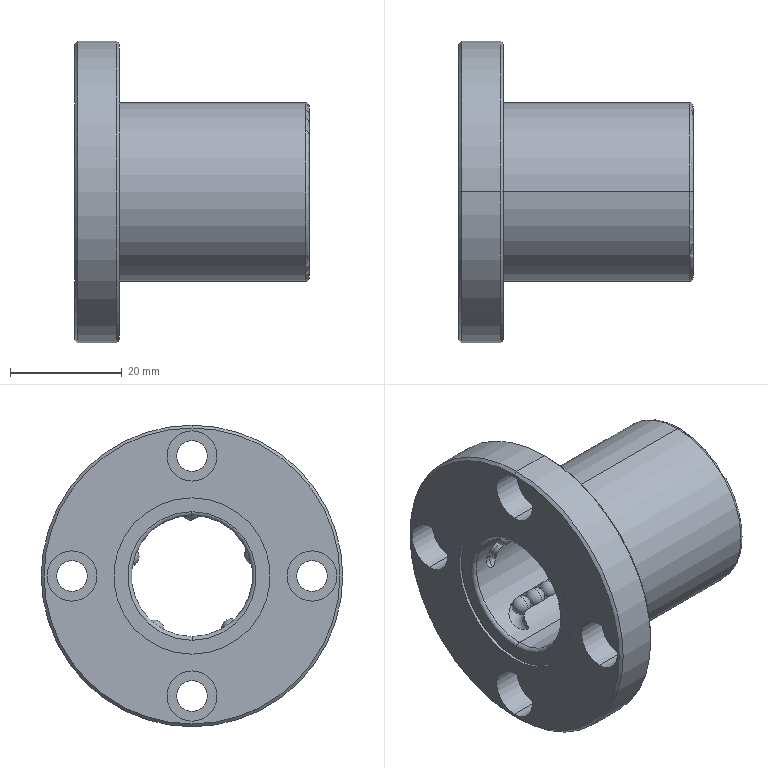Part | STEP file | LMFLMF20UU_LMF6UU | 1 solid | 235 faces | box 42 x 54 x 54 mm | volume 26041 mm3 | cylinder 116 | sphere 80 | torus 26 | plane 9 | cone 4 | commonest cylinder face diameters 3.419 x90 5.5 x8 9 x8 28 x4 21.714 x2 32 x2